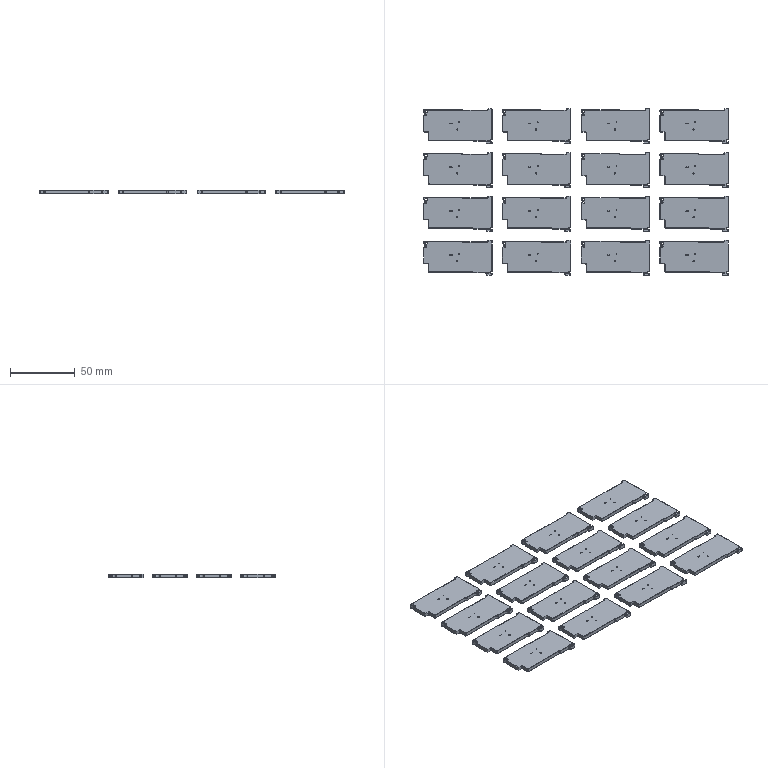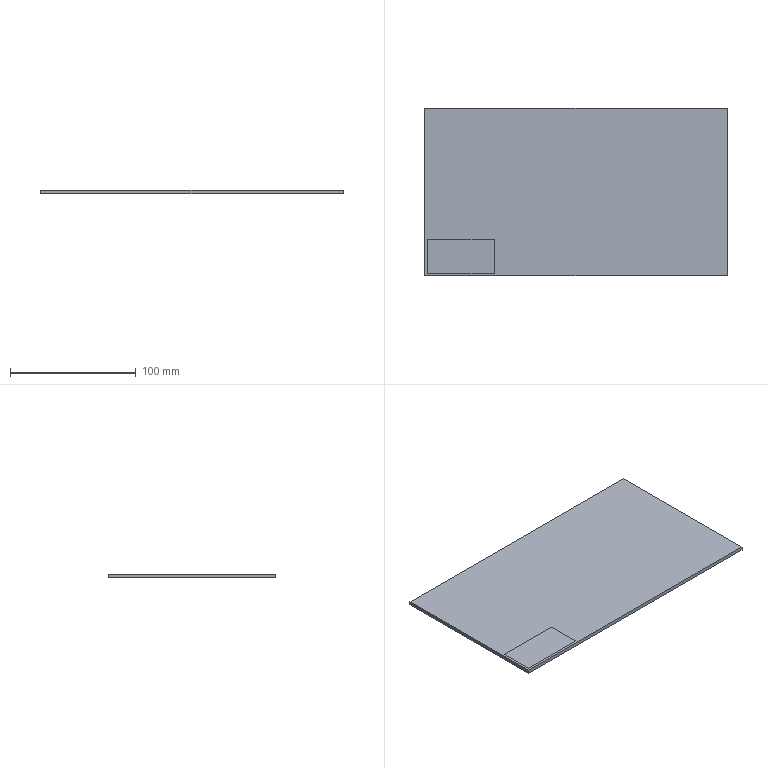CAM job | NX | 3-axis milling, drilling | part box 236.046 x 129.136 x 3 mm | stock box 240.046 x 133.136 x 3 mm
Tools:
number,name,description,diameter,corner_radius,flute_length,length,flutes
3,D3,Milling Tool-5 Parameters,3.0,0.0,50.0,75.0,2
2,D4A45,Milling Tool-5 Parameters,4.0,0.0,2.0,2.0,2
6,D6,Milling Tool-5 Parameters,6.0,0.0,50.0,75.0,2
11,D1,Milling Tool-5 Parameters,1.0,0.0,50.0,75.0,2
18,1.8ZT,Drilling Tool,1.7,0.0,35.0,50.0,2
13,1.1ZT,Drilling Tool,1.0,0.0,35.0,50.0,2
19,0.95ZT,Drilling Tool,0.9,0.0,35.0,50.0,2
16,0.6ZT,Drilling Tool,0.6,0.0,35.0,50.0,2
20,D0.8,Milling Tool-5 Parameters,0.8,0.0,50.0,75.0,2
Operations:
program,operation,operation_type,tool,method,geometry_group,spindle_rpm,surface_speed,feed_per_tooth,feed_cut,feed_plunge,cut_length_mm,path_length_mm,cut_time_min,machine_time_min
1吸,ZLEVEL_PROFILE_COPY_COPY_1_COPY,ZLevelMilling,D6,METHOD,A,9500.0,179.0,0.1158,2200.0,1000.0,17893.828,20698.068,8.461,8.742
1吸,ZLEVEL_PROFILE_COPY_COPY_1_COPY_COPY,ZLevelMilling,D3,METHOD,A,9500.0,89.0,0.0526,1000.0,1000.0,4799.482,17153.503,4.8,6.035
1吸,ZLEVEL_PROFILE_COPY_COPY_1_COPY_COPY_COPY,ZLevelMilling,D1,METHOD,A,9500.0,29.0,0.0447,850.0,1000.0,5681.493,15736.066,6.598,7.604
1吸,ZLEVEL_PROFILE_1_COPY_1_COPY_COPY,ZLevelMilling,D4A45,METHOD,A,9500.0,179.0,0.0526,1000.0,100.0,2723.586,4959.727,2.724,2.947
1吸,ZLEVEL_PROFILE_COPY_COPY_COPY_COPY,ZLevelMilling,D3,MILL_FINISH,A,9500.0,119.0,0.0632,1200.0,1000.0,2734.679,5333.502,2.284,2.544
2,DRILLING_COPY,Operation,D4A45,METHOD,B,5000.0,62.0,0.025,250.0,0.0,25.2,194.875,0.1008,0.1178
2,DRILLING_COPY_COPY_COPY_COPY_COPY,Operation,1.8ZT,METHOD,B,1910.0,21.0,0.0471,180.0,0.0,8.011,76.021,0.0445,0.0513
2,DRILLING_COPY_COPY_COPY_COPY_COPY_COPY,Operation,1.1ZT,METHOD,B,2000.0,6.0,0.025,100.0,0.0,7.8,75.601,0.078,0.0848
2,DRILLING_COPY_COPY_COPY_COPY_COPY_COPY_COPY,Operation,0.95ZT,METHOD,B,2122.0,6.0,0.0165,70.0,0.0,7.77,75.541,0.111,0.1178
2,DRILLING_COPY_COPY_COPY_COPY_COPY_COPY_COPY_COPY,Operation,0.6ZT,METHOD,B,2000.0,3.0,0.0125,50.0,0.0,23.041,121.704,0.4608,0.4707
2,ZLEVEL_PROFILE_COPY_COPY_1_COPY_COPY_1,ZLevelMilling,D0.8,METHOD,B,9500.0,23.0,0.0447,850.0,1000.0,120.096,181.095,0.1378,0.1439
2,ZLEVEL_PROFILE_1_COPY_1_COPY_COPY_COPY,ZLevelMilling,D4A45,METHOD,B,9500.0,179.0,0.0526,1000.0,100.0,169.491,229.491,0.1695,0.1755